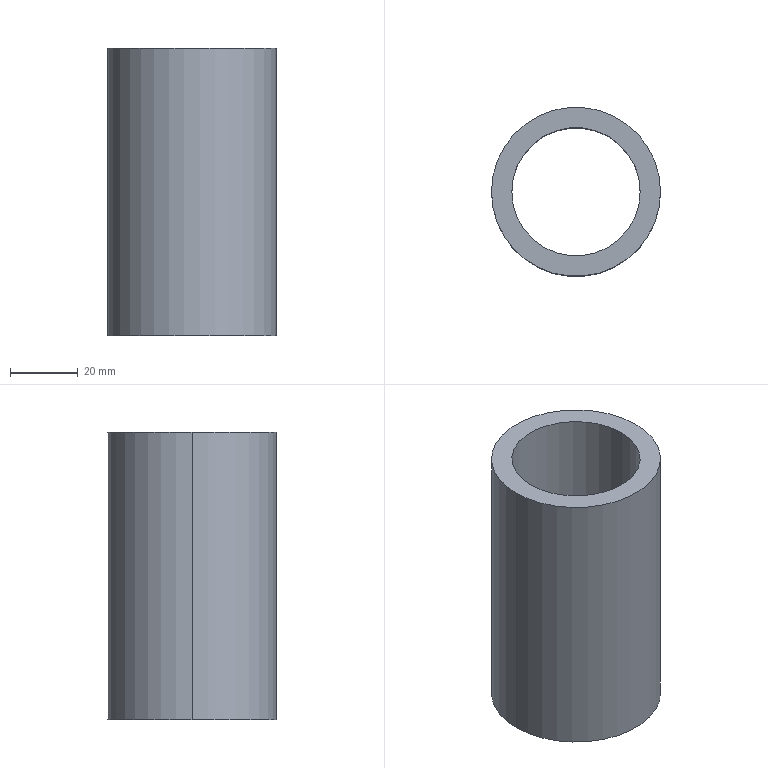Part | STEP file | Nylon centering sleeve SGN-2-32 | 1 solid | 9 faces | box 50 x 50 x 85 mm | volume 68216 mm3 | cylinder 6 | plane 3 | commonest cylinder face diameters 38 x2 45 x2 50 x2
STEP:
#1=CARTESIAN_POINT('',(0.,0.,0.));
#2=DIRECTION('',(0.,0.,1.));
#3=DIRECTION('',(1.,0.,0.));
#4=AXIS2_PLACEMENT_3D('',#1,#2,#3);
#5=CARTESIAN_POINT('',(-22.5,0.,5.));
#6=VERTEX_POINT('',#5);
#7=CARTESIAN_POINT('',(-22.5,0.,0.));
#8=VERTEX_POINT('',#7);
#9=CARTESIAN_POINT('',(-22.5,0.,5.));
#10=DIRECTION('',(0.,0.,-1.));
#11=VECTOR('',#10,1.);
#12=LINE('',#9,#11);
#13=CARTESIAN_POINT('',(0.,0.,5.));
#14=DIRECTION('',(0.,0.,-1.));
#15=DIRECTION('',(-1.,0.,0.));
#16=AXIS2_PLACEMENT_3D('',#13,#14,#15);
#17=CYLINDRICAL_SURFACE('',#16,22.5);
#18=CARTESIAN_POINT('',(6.283,0.));
#19=DIRECTION('',(0.,1.));
#20=VECTOR('',#19,1.);
#21=LINE('',#18,#20);
#22=(GEOMETRIC_REPRESENTATION_CONTEXT(2)PARAMETRIC_REPRESENTATION_CONTEXT()REPRESENTATION_CONTEXT('',''));
#23=DEFINITIONAL_REPRESENTATION('',(#21),#22);
#24=PCURVE('',#17,#23);
#25=CARTESIAN_POINT('',(0.,0.,5.));
#26=DIRECTION('',(0.,0.,-1.));
#27=DIRECTION('',(-1.,0.,0.));
#28=AXIS2_PLACEMENT_3D('',#25,#26,#27);
#29=CYLINDRICAL_SURFACE('',#28,22.5);
#30=CARTESIAN_POINT('',(0.,0.));
#31=DIRECTION('',(0.,1.));
#32=VECTOR('',#31,1.);
#33=LINE('',#30,#32);
#34=(GEOMETRIC_REPRESENTATION_CONTEXT(2)PARAMETRIC_REPRESENTATION_CONTEXT()REPRESENTATION_CONTEXT('',''));
#35=DEFINITIONAL_REPRESENTATION('',(#33),#34);
#36=PCURVE('',#29,#35);
#37=SURFACE_CURVE('',#12,(#24,#36),.PCURVE_S1.);
#38=EDGE_CURVE('',#6,#8,#37,.T.);
#39=ORIENTED_EDGE('',*,*,#38,.T.);
#40=CARTESIAN_POINT('',(22.5,0.,0.));
#41=VERTEX_POINT('',#40);
#42=CARTESIAN_POINT('',(0.,0.,0.));
#43=DIRECTION('',(0.,0.,-1.));
#44=DIRECTION('',(-1.,0.,0.));
#45=AXIS2_PLACEMENT_3D('',#42,#43,#44);
#46=CIRCLE('',#45,22.5);
#47=CARTESIAN_POINT('',(0.,5.));
#48=DIRECTION('',(1.,0.));
#49=VECTOR('',#48,1.);
#50=LINE('',#47,#49);
#51=(GEOMETRIC_REPRESENTATION_CONTEXT(2)PARAMETRIC_REPRESENTATION_CONTEXT()REPRESENTATION_CONTEXT('',''));
#52=DEFINITIONAL_REPRESENTATION('',(#50),#51);
#53=PCURVE('',#17,#52);
#54=CARTESIAN_POINT('',(0.,0.,0.));
#55=DIRECTION('',(0.,0.,1.));
#56=DIRECTION('',(1.,0.,0.));
#57=AXIS2_PLACEMENT_3D('',#54,#55,#56);
#58=PLANE('',#57);
#59=CARTESIAN_POINT('',(-22.5,0.));
#60=CARTESIAN_POINT('',(-22.5,38.971));
#61=CARTESIAN_POINT('',(11.25,19.486));
#62=CARTESIAN_POINT('',(45.,0.));
#63=CARTESIAN_POINT('',(11.25,-19.486));
#64=CARTESIAN_POINT('',(-22.5,-38.971));
#65=CARTESIAN_POINT('',(-22.5,0.));
#66=(BOUNDED_CURVE()B_SPLINE_CURVE(2,(#59,#60,#61,#62,#63,#64,#65),.UNSPECIFIED.,.T.,.F.)B_SPLINE_CURVE_WITH_KNOTS((1,2,2,2,2,1),(-2.094,0.,2.094,4.189,6.283,8.378),.UNSPECIFIED.)CURVE()GEOMETRIC_REPRESENTATION_ITEM()RATIONAL_B_SPLINE_CURVE((1.,0.5,1.,0.5,1.,0.5,1.))REPRESENTATION_ITEM(''));
#67=(GEOMETRIC_REPRESENTATION_CONTEXT(2)PARAMETRIC_REPRESENTATION_CONTEXT()REPRESENTATION_CONTEXT('',''));
#68=DEFINITIONAL_REPRESENTATION('',(#66),#67);
#69=PCURVE('',#58,#68);
#70=SURFACE_CURVE('',#46,(#53,#69),.PCURVE_S1.);
#71=EDGE_CURVE('',#41,#8,#70,.T.);
#72=ORIENTED_EDGE('',*,*,#71,.F.);
#73=CARTESIAN_POINT('',(22.5,0.,5.));
#74=VERTEX_POINT('',#73);
#75=CARTESIAN_POINT('',(22.5,0.,5.));
#76=DIRECTION('',(0.,0.,-1.));
#77=VECTOR('',#76,1.);
#78=LINE('',#75,#77);
#79=CARTESIAN_POINT('',(3.142,0.));
#80=DIRECTION('',(0.,1.));
#81=VECTOR('',#80,1.);
#82=LINE('',#79,#81);
#83=(GEOMETRIC_REPRESENTATION_CONTEXT(2)PARAMETRIC_REPRESENTATION_CONTEXT()REPRESENTATION_CONTEXT('',''));
#84=DEFINITIONAL_REPRESENTATION('',(#82),#83);
#85=PCURVE('',#17,#84);
#86=CARTESIAN_POINT('',(3.142,0.));
#87=DIRECTION('',(0.,1.));
#88=VECTOR('',#87,1.);
#89=LINE('',#86,#88);
#90=(GEOMETRIC_REPRESENTATION_CONTEXT(2)PARAMETRIC_REPRESENTATION_CONTEXT()REPRESENTATION_CONTEXT('',''));
#91=DEFINITIONAL_REPRESENTATION('',(#89),#90);
#92=PCURVE('',#29,#91);
#93=SURFACE_CURVE('',#78,(#85,#92),.PCURVE_S1.);
#94=EDGE_CURVE('',#74,#41,#93,.T.);
#95=ORIENTED_EDGE('',*,*,#94,.F.);
#96=CARTESIAN_POINT('',(0.,0.,5.));
#97=DIRECTION('',(0.,0.,-1.));
#98=DIRECTION('',(-1.,0.,0.));
#99=AXIS2_PLACEMENT_3D('',#96,#97,#98);
#100=CIRCLE('',#99,22.5);
#101=CARTESIAN_POINT('',(0.,0.));
#102=DIRECTION('',(1.,0.));
#103=VECTOR('',#102,1.);
#104=LINE('',#101,#103);
#105=(GEOMETRIC_REPRESENTATION_CONTEXT(2)PARAMETRIC_REPRESENTATION_CONTEXT()REPRESENTATION_CONTEXT('',''));
#106=DEFINITIONAL_REPRESENTATION('',(#104),#105);
#107=PCURVE('',#17,#106);
#108=CARTESIAN_POINT('',(0.,0.,5.));
#109=DIRECTION('',(0.,0.,-1.));
#110=DIRECTION('',(-1.,0.,0.));
#111=AXIS2_PLACEMENT_3D('',#108,#109,#110);
#112=PLANE('',#111);
#113=CARTESIAN_POINT('',(0.,0.));
#114=DIRECTION('',(1.,0.));
#115=AXIS2_PLACEMENT_2D('',#113,#114);
#116=CIRCLE('',#115,22.5);
#117=(GEOMETRIC_REPRESENTATION_CONTEXT(2)PARAMETRIC_REPRESENTATION_CONTEXT()REPRESENTATION_CONTEXT('',''));
#118=DEFINITIONAL_REPRESENTATION('',(#116),#117);
#119=PCURVE('',#112,#118);
#120=SURFACE_CURVE('',#100,(#107,#119),.PCURVE_S1.);
#121=EDGE_CURVE('',#74,#6,#120,.T.);
#122=ORIENTED_EDGE('',*,*,#121,.T.);
#123=EDGE_LOOP('',(#39,#72,#95,#122));
#124=FACE_BOUND('',#123,.F.);
#125=ADVANCED_FACE('',(#124),#17,.F.);
#126=CARTESIAN_POINT('',(25.,0.,85.));
#127=VERTEX_POINT('',#126);
#128=CARTESIAN_POINT('',(-25.,0.,85.));
#129=VERTEX_POINT('',#128);
#130=CARTESIAN_POINT('',(0.,0.,85.));
#131=DIRECTION('',(0.,0.,1.));
#132=DIRECTION('',(1.,0.,0.));
#133=AXIS2_PLACEMENT_3D('',#130,#131,#132);
#134=CIRCLE('',#133,25.);
#135=CARTESIAN_POINT('',(0.,0.,85.));
#136=DIRECTION('',(0.,0.,-1.));
#137=DIRECTION('',(-1.,0.,0.));
#138=AXIS2_PLACEMENT_3D('',#135,#136,#137);
#139=CYLINDRICAL_SURFACE('',#138,25.);
#140=CARTESIAN_POINT('',(3.142,0.));
#141=DIRECTION('',(-1.,0.));
#142=VECTOR('',#141,1.);
#143=LINE('',#140,#142);
#144=(GEOMETRIC_REPRESENTATION_CONTEXT(2)PARAMETRIC_REPRESENTATION_CONTEXT()REPRESENTATION_CONTEXT('',''));
#145=DEFINITIONAL_REPRESENTATION('',(#143),#144);
#146=PCURVE('',#139,#145);
#147=CARTESIAN_POINT('',(0.,0.,85.));
#148=DIRECTION('',(0.,0.,1.));
#149=DIRECTION('',(1.,0.,0.));
#150=AXIS2_PLACEMENT_3D('',#147,#148,#149);
#151=PLANE('',#150);
#152=CARTESIAN_POINT('',(0.,0.));
#153=DIRECTION('',(1.,0.));
#154=AXIS2_PLACEMENT_2D('',#152,#153);
#155=CIRCLE('',#154,25.);
#156=(GEOMETRIC_REPRESENTATION_CONTEXT(2)PARAMETRIC_REPRESENTATION_CONTEXT()REPRESENTATION_CONTEXT('',''));
#157=DEFINITIONAL_REPRESENTATION('',(#155),#156);
#158=PCURVE('',#151,#157);
#159=SURFACE_CURVE('',#134,(#146,#158),.PCURVE_S1.);
#160=EDGE_CURVE('',#127,#129,#159,.T.);
#161=ORIENTED_EDGE('',*,*,#160,.F.);
#162=CARTESIAN_POINT('',(25.,0.,0.));
#163=VERTEX_POINT('',#162);
#164=CARTESIAN_POINT('',(25.,0.,85.));
#165=DIRECTION('',(0.,0.,-1.));
#166=VECTOR('',#165,1.);
#167=LINE('',#164,#166);
#168=CARTESIAN_POINT('',(3.142,0.));
#169=DIRECTION('',(0.,1.));
#170=VECTOR('',#169,1.);
#171=LINE('',#168,#170);
#172=(GEOMETRIC_REPRESENTATION_CONTEXT(2)PARAMETRIC_REPRESENTATION_CONTEXT()REPRESENTATION_CONTEXT('',''));
#173=DEFINITIONAL_REPRESENTATION('',(#171),#172);
#174=PCURVE('',#139,#173);
#175=CARTESIAN_POINT('',(0.,0.,85.));
#176=DIRECTION('',(0.,0.,-1.));
#177=DIRECTION('',(-1.,0.,0.));
#178=AXIS2_PLACEMENT_3D('',#175,#176,#177);
#179=CYLINDRICAL_SURFACE('',#178,25.);
#180=CARTESIAN_POINT('',(3.142,0.));
#181=DIRECTION('',(0.,1.));
#182=VECTOR('',#181,1.);
#183=LINE('',#180,#182);
#184=(GEOMETRIC_REPRESENTATION_CONTEXT(2)PARAMETRIC_REPRESENTATION_CONTEXT()REPRESENTATION_CONTEXT('',''));
#185=DEFINITIONAL_REPRESENTATION('',(#183),#184);
#186=PCURVE('',#179,#185);
#187=SURFACE_CURVE('',#167,(#174,#186),.PCURVE_S1.);
#188=EDGE_CURVE('',#127,#163,#187,.T.);
#189=ORIENTED_EDGE('',*,*,#188,.T.);
#190=CARTESIAN_POINT('',(-25.,0.,0.));
#191=VERTEX_POINT('',#190);
#192=CARTESIAN_POINT('',(0.,0.,0.));
#193=DIRECTION('',(0.,0.,1.));
#194=DIRECTION('',(1.,0.,0.));
#195=AXIS2_PLACEMENT_3D('',#192,#193,#194);
#196=CIRCLE('',#195,25.);
#197=CARTESIAN_POINT('',(3.142,85.));
#198=DIRECTION('',(-1.,0.));
#199=VECTOR('',#198,1.);
#200=LINE('',#197,#199);
#201=(GEOMETRIC_REPRESENTATION_CONTEXT(2)PARAMETRIC_REPRESENTATION_CONTEXT()REPRESENTATION_CONTEXT('',''));
#202=DEFINITIONAL_REPRESENTATION('',(#200),#201);
#203=PCURVE('',#139,#202);
#204=CARTESIAN_POINT('',(0.,0.));
#205=DIRECTION('',(1.,0.));
#206=AXIS2_PLACEMENT_2D('',#204,#205);
#207=CIRCLE('',#206,25.);
#208=(GEOMETRIC_REPRESENTATION_CONTEXT(2)PARAMETRIC_REPRESENTATION_CONTEXT()REPRESENTATION_CONTEXT('',''));
#209=DEFINITIONAL_REPRESENTATION('',(#207),#208);
#210=PCURVE('',#58,#209);
#211=SURFACE_CURVE('',#196,(#203,#210),.PCURVE_S1.);
#212=EDGE_CURVE('',#163,#191,#211,.T.);
#213=ORIENTED_EDGE('',*,*,#212,.T.);
#214=CARTESIAN_POINT('',(-25.,0.,85.));
#215=DIRECTION('',(0.,0.,-1.));
#216=VECTOR('',#215,1.);
#217=LINE('',#214,#216);
#218=CARTESIAN_POINT('',(0.,0.));
#219=DIRECTION('',(0.,1.));
#220=VECTOR('',#219,1.);
#221=LINE('',#218,#220);
#222=(GEOMETRIC_REPRESENTATION_CONTEXT(2)PARAMETRIC_REPRESENTATION_CONTEXT()REPRESENTATION_CONTEXT('',''));
#223=DEFINITIONAL_REPRESENTATION('',(#221),#222);
#224=PCURVE('',#139,#223);
#225=CARTESIAN_POINT('',(6.283,0.));
#226=DIRECTION('',(0.,1.));
#227=VECTOR('',#226,1.);
#228=LINE('',#225,#227);
#229=(GEOMETRIC_REPRESENTATION_CONTEXT(2)PARAMETRIC_REPRESENTATION_CONTEXT()REPRESENTATION_CONTEXT('',''));
#230=DEFINITIONAL_REPRESENTATION('',(#228),#229);
#231=PCURVE('',#179,#230);
#232=SURFACE_CURVE('',#217,(#224,#231),.PCURVE_S1.);
#233=EDGE_CURVE('',#129,#191,#232,.T.);
#234=ORIENTED_EDGE('',*,*,#233,.F.);
#235=EDGE_LOOP('',(#161,#189,#213,#234));
#236=FACE_BOUND('',#235,.T.);
#237=ADVANCED_FACE('',(#236),#139,.T.);
#238=CARTESIAN_POINT('',(-19.,0.,85.));
#239=VERTEX_POINT('',#238);
#240=CARTESIAN_POINT('',(-19.,0.,5.));
#241=VERTEX_POINT('',#240);
#242=CARTESIAN_POINT('',(-19.,0.,85.));
#243=DIRECTION('',(0.,0.,-1.));
#244=VECTOR('',#243,1.);
#245=LINE('',#242,#244);
#246=CARTESIAN_POINT('',(0.,0.,85.));
#247=DIRECTION('',(0.,0.,-1.));
#248=DIRECTION('',(-1.,0.,0.));
#249=AXIS2_PLACEMENT_3D('',#246,#247,#248);
#250=CYLINDRICAL_SURFACE('',#249,19.);
#251=CARTESIAN_POINT('',(6.283,0.));
#252=DIRECTION('',(0.,1.));
#253=VECTOR('',#252,1.);
#254=LINE('',#251,#253);
#255=(GEOMETRIC_REPRESENTATION_CONTEXT(2)PARAMETRIC_REPRESENTATION_CONTEXT()REPRESENTATION_CONTEXT('',''));
#256=DEFINITIONAL_REPRESENTATION('',(#254),#255);
#257=PCURVE('',#250,#256);
#258=CARTESIAN_POINT('',(0.,0.,85.));
#259=DIRECTION('',(0.,0.,-1.));
#260=DIRECTION('',(-1.,0.,0.));
#261=AXIS2_PLACEMENT_3D('',#258,#259,#260);
#262=CYLINDRICAL_SURFACE('',#261,19.);
#263=CARTESIAN_POINT('',(0.,0.));
#264=DIRECTION('',(0.,1.));
#265=VECTOR('',#264,1.);
#266=LINE('',#263,#265);
#267=(GEOMETRIC_REPRESENTATION_CONTEXT(2)PARAMETRIC_REPRESENTATION_CONTEXT()REPRESENTATION_CONTEXT('',''));
#268=DEFINITIONAL_REPRESENTATION('',(#266),#267);
#269=PCURVE('',#262,#268);
#270=SURFACE_CURVE('',#245,(#257,#269),.PCURVE_S1.);
#271=EDGE_CURVE('',#239,#241,#270,.T.);
#272=ORIENTED_EDGE('',*,*,#271,.T.);
#273=CARTESIAN_POINT('',(19.,0.,5.));
#274=VERTEX_POINT('',#273);
#275=CARTESIAN_POINT('',(0.,0.,5.));
#276=DIRECTION('',(0.,0.,-1.));
#277=DIRECTION('',(-1.,0.,0.));
#278=AXIS2_PLACEMENT_3D('',#275,#276,#277);
#279=CIRCLE('',#278,19.);
#280=CARTESIAN_POINT('',(0.,80.));
#281=DIRECTION('',(1.,0.));
#282=VECTOR('',#281,1.);
#283=LINE('',#280,#282);
#284=(GEOMETRIC_REPRESENTATION_CONTEXT(2)PARAMETRIC_REPRESENTATION_CONTEXT()REPRESENTATION_CONTEXT('',''));
#285=DEFINITIONAL_REPRESENTATION('',(#283),#284);
#286=PCURVE('',#250,#285);
#287=CARTESIAN_POINT('',(0.,0.));
#288=DIRECTION('',(1.,0.));
#289=AXIS2_PLACEMENT_2D('',#287,#288);
#290=CIRCLE('',#289,19.);
#291=(GEOMETRIC_REPRESENTATION_CONTEXT(2)PARAMETRIC_REPRESENTATION_CONTEXT()REPRESENTATION_CONTEXT('',''));
#292=DEFINITIONAL_REPRESENTATION('',(#290),#291);
#293=PCURVE('',#112,#292);
#294=SURFACE_CURVE('',#279,(#286,#293),.PCURVE_S1.);
#295=EDGE_CURVE('',#274,#241,#294,.T.);
#296=ORIENTED_EDGE('',*,*,#295,.F.);
#297=CARTESIAN_POINT('',(19.,0.,85.));
#298=VERTEX_POINT('',#297);
#299=CARTESIAN_POINT('',(19.,0.,85.));
#300=DIRECTION('',(0.,0.,-1.));
#301=VECTOR('',#300,1.);
#302=LINE('',#299,#301);
#303=CARTESIAN_POINT('',(3.142,0.));
#304=DIRECTION('',(0.,1.));
#305=VECTOR('',#304,1.);
#306=LINE('',#303,#305);
#307=(GEOMETRIC_REPRESENTATION_CONTEXT(2)PARAMETRIC_REPRESENTATION_CONTEXT()REPRESENTATION_CONTEXT('',''));
#308=DEFINITIONAL_REPRESENTATION('',(#306),#307);
#309=PCURVE('',#250,#308);
#310=CARTESIAN_POINT('',(3.142,0.));
#311=DIRECTION('',(0.,1.));
#312=VECTOR('',#311,1.);
#313=LINE('',#310,#312);
#314=(GEOMETRIC_REPRESENTATION_CONTEXT(2)PARAMETRIC_REPRESENTATION_CONTEXT()REPRESENTATION_CONTEXT('',''));
#315=DEFINITIONAL_REPRESENTATION('',(#313),#314);
#316=PCURVE('',#262,#315);
#317=SURFACE_CURVE('',#302,(#309,#316),.PCURVE_S1.);
#318=EDGE_CURVE('',#298,#274,#317,.T.);
#319=ORIENTED_EDGE('',*,*,#318,.F.);
#320=CARTESIAN_POINT('',(0.,0.,85.));
#321=DIRECTION('',(0.,0.,1.));
#322=DIRECTION('',(1.,0.,0.));
#323=AXIS2_PLACEMENT_3D('',#320,#321,#322);
#324=CIRCLE('',#323,19.);
#325=CARTESIAN_POINT('',(9.425,0.));
#326=DIRECTION('',(-1.,0.));
#327=VECTOR('',#326,1.);
#328=LINE('',#325,#327);
#329=(GEOMETRIC_REPRESENTATION_CONTEXT(2)PARAMETRIC_REPRESENTATION_CONTEXT()REPRESENTATION_CONTEXT('',''));
#330=DEFINITIONAL_REPRESENTATION('',(#328),#329);
#331=PCURVE('',#250,#330);
#332=CARTESIAN_POINT('',(0.,0.));
#333=DIRECTION('',(1.,0.));
#334=AXIS2_PLACEMENT_2D('',#332,#333);
#335=CIRCLE('',#334,19.);
#336=(GEOMETRIC_REPRESENTATION_CONTEXT(2)PARAMETRIC_REPRESENTATION_CONTEXT()REPRESENTATION_CONTEXT('',''));
#337=DEFINITIONAL_REPRESENTATION('',(#335),#336);
#338=PCURVE('',#151,#337);
#339=SURFACE_CURVE('',#324,(#331,#338),.PCURVE_S1.);
#340=EDGE_CURVE('',#239,#298,#339,.T.);
#341=ORIENTED_EDGE('',*,*,#340,.F.);
#342=EDGE_LOOP('',(#272,#296,#319,#341));
#343=FACE_BOUND('',#342,.F.);
#344=ADVANCED_FACE('',(#343),#250,.F.);
#345=CARTESIAN_POINT('',(0.,0.,5.));
#346=DIRECTION('',(0.,0.,-1.));
#347=DIRECTION('',(-1.,0.,0.));
#348=AXIS2_PLACEMENT_3D('',#345,#346,#347);
#349=CIRCLE('',#348,19.);
#350=CARTESIAN_POINT('',(0.,80.));
#351=DIRECTION('',(1.,0.));
#352=VECTOR('',#351,1.);
#353=LINE('',#350,#352);
#354=(GEOMETRIC_REPRESENTATION_CONTEXT(2)PARAMETRIC_REPRESENTATION_CONTEXT()REPRESENTATION_CONTEXT('',''));
#355=DEFINITIONAL_REPRESENTATION('',(#353),#354);
#356=PCURVE('',#262,#355);
#357=CARTESIAN_POINT('',(0.,0.));
#358=DIRECTION('',(1.,0.));
#359=AXIS2_PLACEMENT_2D('',#357,#358);
#360=CIRCLE('',#359,19.);
#361=(GEOMETRIC_REPRESENTATION_CONTEXT(2)PARAMETRIC_REPRESENTATION_CONTEXT()REPRESENTATION_CONTEXT('',''));
#362=DEFINITIONAL_REPRESENTATION('',(#360),#361);
#363=PCURVE('',#112,#362);
#364=SURFACE_CURVE('',#349,(#356,#363),.PCURVE_S1.);
#365=EDGE_CURVE('',#241,#274,#364,.T.);
#366=ORIENTED_EDGE('',*,*,#365,.F.);
#367=ORIENTED_EDGE('',*,*,#271,.F.);
#368=CARTESIAN_POINT('',(0.,0.,85.));
#369=DIRECTION('',(0.,0.,1.));
#370=DIRECTION('',(1.,0.,0.));
#371=AXIS2_PLACEMENT_3D('',#368,#369,#370);
#372=CIRCLE('',#371,19.);
#373=CARTESIAN_POINT('',(3.142,0.));
#374=DIRECTION('',(-1.,0.));
#375=VECTOR('',#374,1.);
#376=LINE('',#373,#375);
#377=(GEOMETRIC_REPRESENTATION_CONTEXT(2)PARAMETRIC_REPRESENTATION_CONTEXT()REPRESENTATION_CONTEXT('',''));
#378=DEFINITIONAL_REPRESENTATION('',(#376),#377);
#379=PCURVE('',#262,#378);
#380=CARTESIAN_POINT('',(0.,0.));
#381=DIRECTION('',(1.,0.));
#382=AXIS2_PLACEMENT_2D('',#380,#381);
#383=CIRCLE('',#382,19.);
#384=(GEOMETRIC_REPRESENTATION_CONTEXT(2)PARAMETRIC_REPRESENTATION_CONTEXT()REPRESENTATION_CONTEXT('',''));
#385=DEFINITIONAL_REPRESENTATION('',(#383),#384);
#386=PCURVE('',#151,#385);
#387=SURFACE_CURVE('',#372,(#379,#386),.PCURVE_S1.);
#388=EDGE_CURVE('',#298,#239,#387,.T.);
#389=ORIENTED_EDGE('',*,*,#388,.F.);
#390=ORIENTED_EDGE('',*,*,#318,.T.);
#391=EDGE_LOOP('',(#366,#367,#389,#390));
#392=FACE_BOUND('',#391,.F.);
#393=ADVANCED_FACE('',(#392),#262,.F.);
#394=CARTESIAN_POINT('',(0.,0.,85.));
#395=DIRECTION('',(0.,0.,1.));
#396=DIRECTION('',(1.,0.,0.));
#397=AXIS2_PLACEMENT_3D('',#394,#395,#396);
#398=CIRCLE('',#397,25.);
#399=CARTESIAN_POINT('',(0.,0.));
#400=DIRECTION('',(1.,0.));
#401=AXIS2_PLACEMENT_2D('',#399,#400);
#402=CIRCLE('',#401,25.);
#403=(GEOMETRIC_REPRESENTATION_CONTEXT(2)PARAMETRIC_REPRESENTATION_CONTEXT()REPRESENTATION_CONTEXT('',''));
#404=DEFINITIONAL_REPRESENTATION('',(#402),#403);
#405=PCURVE('',#151,#404);
#406=CARTESIAN_POINT('',(9.425,0.));
#407=DIRECTION('',(-1.,0.));
#408=VECTOR('',#407,1.);
#409=LINE('',#406,#408);
#410=(GEOMETRIC_REPRESENTATION_CONTEXT(2)PARAMETRIC_REPRESENTATION_CONTEXT()REPRESENTATION_CONTEXT('',''));
#411=DEFINITIONAL_REPRESENTATION('',(#409),#410);
#412=PCURVE('',#179,#411);
#413=SURFACE_CURVE('',#398,(#405,#412),.PCURVE_S1.);
#414=EDGE_CURVE('',#129,#127,#413,.T.);
#415=ORIENTED_EDGE('',*,*,#414,.T.);
#416=ORIENTED_EDGE('',*,*,#160,.T.);
#417=EDGE_LOOP('',(#415,#416));
#418=FACE_BOUND('',#417,.T.);
#419=ORIENTED_EDGE('',*,*,#340,.F.);
#420=ORIENTED_EDGE('',*,*,#388,.F.);
#421=EDGE_LOOP('',(#419,#420));
#422=FACE_BOUND('',#421,.T.);
#423=ADVANCED_FACE('',(#418,#422),#151,.T.);
#424=CARTESIAN_POINT('',(0.,0.,0.));
#425=DIRECTION('',(0.,0.,-1.));
#426=DIRECTION('',(-1.,0.,0.));
#427=AXIS2_PLACEMENT_3D('',#424,#425,#426);
#428=CIRCLE('',#427,22.5);
#429=CARTESIAN_POINT('',(-22.5,0.));
#430=CARTESIAN_POINT('',(-22.5,38.971));
#431=CARTESIAN_POINT('',(11.25,19.486));
#432=CARTESIAN_POINT('',(45.,0.));
#433=CARTESIAN_POINT('',(11.25,-19.486));
#434=CARTESIAN_POINT('',(-22.5,-38.971));
#435=CARTESIAN_POINT('',(-22.5,0.));
#436=(BOUNDED_CURVE()B_SPLINE_CURVE(2,(#429,#430,#431,#432,#433,#434,#435),.UNSPECIFIED.,.T.,.F.)B_SPLINE_CURVE_WITH_KNOTS((1,2,2,2,2,1),(-2.094,0.,2.094,4.189,6.283,8.378),.UNSPECIFIED.)CURVE()GEOMETRIC_REPRESENTATION_ITEM()RATIONAL_B_SPLINE_CURVE((1.,0.5,1.,0.5,1.,0.5,1.))REPRESENTATION_ITEM(''));
#437=(GEOMETRIC_REPRESENTATION_CONTEXT(2)PARAMETRIC_REPRESENTATION_CONTEXT()REPRESENTATION_CONTEXT('',''));
#438=DEFINITIONAL_REPRESENTATION('',(#436),#437);
#439=PCURVE('',#58,#438);
#440=CARTESIAN_POINT('',(0.,5.));
#441=DIRECTION('',(1.,0.));
#442=VECTOR('',#441,1.);
#443=LINE('',#440,#442);
#444=(GEOMETRIC_REPRESENTATION_CONTEXT(2)PARAMETRIC_REPRESENTATION_CONTEXT()REPRESENTATION_CONTEXT('',''));
#445=DEFINITIONAL_REPRESENTATION('',(#443),#444);
#446=PCURVE('',#29,#445);
#447=SURFACE_CURVE('',#428,(#439,#446),.PCURVE_S1.);
#448=EDGE_CURVE('',#8,#41,#447,.T.);
#449=ORIENTED_EDGE('',*,*,#448,.F.);
#450=ORIENTED_EDGE('',*,*,#71,.F.);
#451=EDGE_LOOP('',(#449,#450));
#452=FACE_BOUND('',#451,.T.);
#453=CARTESIAN_POINT('',(0.,0.,0.));
#454=DIRECTION('',(0.,0.,1.));
#455=DIRECTION('',(1.,0.,0.));
#456=AXIS2_PLACEMENT_3D('',#453,#454,#455);
#457=CIRCLE('',#456,25.);
#458=CARTESIAN_POINT('',(0.,0.));
#459=DIRECTION('',(1.,0.));
#460=AXIS2_PLACEMENT_2D('',#458,#459);
#461=CIRCLE('',#460,25.);
#462=(GEOMETRIC_REPRESENTATION_CONTEXT(2)PARAMETRIC_REPRESENTATION_CONTEXT()REPRESENTATION_CONTEXT('',''));
#463=DEFINITIONAL_REPRESENTATION('',(#461),#462);
#464=PCURVE('',#58,#463);
#465=CARTESIAN_POINT('',(9.425,85.));
#466=DIRECTION('',(-1.,0.));
#467=VECTOR('',#466,1.);
#468=LINE('',#465,#467);
#469=(GEOMETRIC_REPRESENTATION_CONTEXT(2)PARAMETRIC_REPRESENTATION_CONTEXT()REPRESENTATION_CONTEXT('',''));
#470=DEFINITIONAL_REPRESENTATION('',(#468),#469);
#471=PCURVE('',#179,#470);
#472=SURFACE_CURVE('',#457,(#464,#471),.PCURVE_S1.);
#473=EDGE_CURVE('',#191,#163,#472,.T.);
#474=ORIENTED_EDGE('',*,*,#473,.F.);
#475=ORIENTED_EDGE('',*,*,#212,.F.);
#476=EDGE_LOOP('',(#474,#475));
#477=FACE_BOUND('',#476,.T.);
#478=ADVANCED_FACE('',(#452,#477),#58,.F.);
#479=ORIENTED_EDGE('',*,*,#188,.F.);
#480=ORIENTED_EDGE('',*,*,#414,.F.);
#481=ORIENTED_EDGE('',*,*,#233,.T.);
#482=ORIENTED_EDGE('',*,*,#473,.T.);
#483=EDGE_LOOP('',(#479,#480,#481,#482));
#484=FACE_BOUND('',#483,.T.);
#485=ADVANCED_FACE('',(#484),#179,.T.);
#486=ORIENTED_EDGE('',*,*,#448,.F.);
#487=ORIENTED_EDGE('',*,*,#38,.F.);
#488=CARTESIAN_POINT('',(0.,0.,5.));
#489=DIRECTION('',(0.,0.,-1.));
#490=DIRECTION('',(-1.,0.,0.));
#491=AXIS2_PLACEMENT_3D('',#488,#489,#490);
#492=CIRCLE('',#491,22.5);
#493=CARTESIAN_POINT('',(0.,0.));
#494=DIRECTION('',(1.,0.));
#495=VECTOR('',#494,1.);
#496=LINE('',#493,#495);
#497=(GEOMETRIC_REPRESENTATION_CONTEXT(2)PARAMETRIC_REPRESENTATION_CONTEXT()REPRESENTATION_CONTEXT('',''));
#498=DEFINITIONAL_REPRESENTATION('',(#496),#497);
#499=PCURVE('',#29,#498);
#500=CARTESIAN_POINT('',(0.,0.));
#501=DIRECTION('',(1.,0.));
#502=AXIS2_PLACEMENT_2D('',#500,#501);
#503=CIRCLE('',#502,22.5);
#504=(GEOMETRIC_REPRESENTATION_CONTEXT(2)PARAMETRIC_REPRESENTATION_CONTEXT()REPRESENTATION_CONTEXT('',''));
#505=DEFINITIONAL_REPRESENTATION('',(#503),#504);
#506=PCURVE('',#112,#505);
#507=SURFACE_CURVE('',#492,(#499,#506),.PCURVE_S1.);
#508=EDGE_CURVE('',#6,#74,#507,.T.);
#509=ORIENTED_EDGE('',*,*,#508,.T.);
#510=ORIENTED_EDGE('',*,*,#94,.T.);
#511=EDGE_LOOP('',(#486,#487,#509,#510));
#512=FACE_BOUND('',#511,.F.);
#513=ADVANCED_FACE('',(#512),#29,.F.);
#514=ORIENTED_EDGE('',*,*,#365,.F.);
#515=ORIENTED_EDGE('',*,*,#295,.F.);
#516=EDGE_LOOP('',(#514,#515));
#517=FACE_BOUND('',#516,.T.);
#518=ORIENTED_EDGE('',*,*,#508,.T.);
#519=ORIENTED_EDGE('',*,*,#121,.T.);
#520=EDGE_LOOP('',(#518,#519));
#521=FACE_BOUND('',#520,.T.);
#522=ADVANCED_FACE('',(#517,#521),#112,.T.);
#523=CLOSED_SHELL('',(#125,#237,#344,#393,#423,#478,#485,#513,#522));
#524=MANIFOLD_SOLID_BREP('',#523);
#525=(LENGTH_UNIT()NAMED_UNIT(*)SI_UNIT(.MILLI.,.METRE.));
#526=UNCERTAINTY_MEASURE_WITH_UNIT(LENGTH_MEASURE(0.0000001),#525,'','');
#527=(NAMED_UNIT(*)PLANE_ANGLE_UNIT()SI_UNIT($,.RADIAN.));
#528=(NAMED_UNIT(*)SI_UNIT($,.STERADIAN.)SOLID_ANGLE_UNIT());
#529=(GEOMETRIC_REPRESENTATION_CONTEXT(3)GLOBAL_UNCERTAINTY_ASSIGNED_CONTEXT((#526))GLOBAL_UNIT_ASSIGNED_CONTEXT((#525,#527,#528))REPRESENTATION_CONTEXT('',''));
#530=ADVANCED_BREP_SHAPE_REPRESENTATION('',(#4,#524),#529);